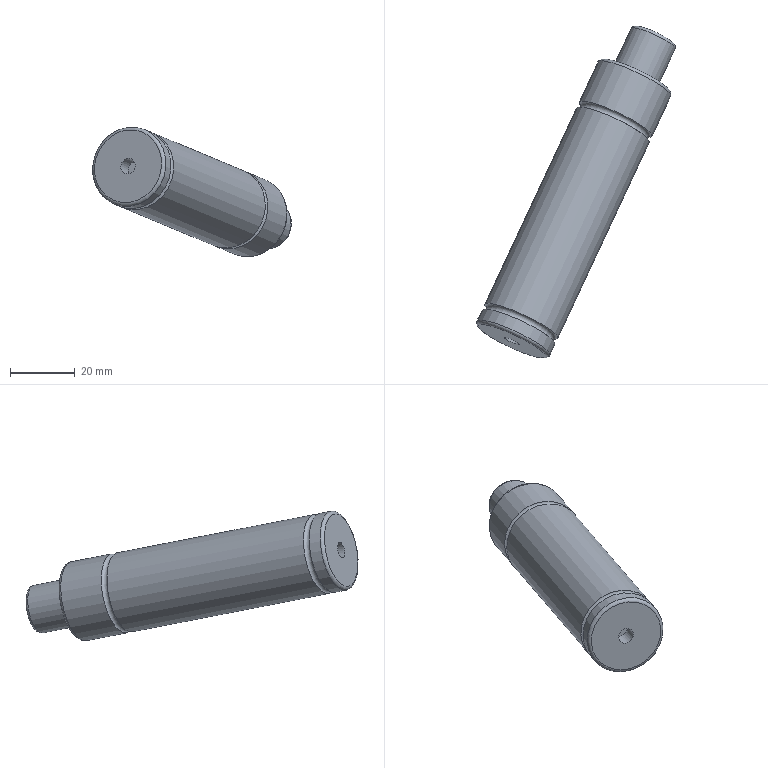Part | NX | features 1 2 | 1 solid | 17 faces | box 61.606 x 102.919 x 40.18 mm | volume 46865 mm3 | cylinder 6 | torus 5 | plane 4 | cone 2 | commonest cylinder face diameters 24.9 x3 2 x1 4.9 x1 15 x1
STEP:
#1=CARTESIAN_POINT('',(294.815,638.267,112.369));
#2=VERTEX_POINT('',#1);
#3=CARTESIAN_POINT('',(283.532,643.529,112.369));
#4=DIRECTION('',(0.4162,0.8925,-0.1736));
#5=DIRECTION('',(0.9063,-0.4226,0.));
#6=AXIS2_PLACEMENT_3D('',#3,#4,#5);
#7=CIRCLE('',#6,12.45);
#8=EDGE_CURVE('',#2,#2,#7,.T.);
#9=ORIENTED_EDGE('',*,*,#8,.T.);
#10=EDGE_LOOP('',(#9));
#11=FACE_BOUND('',#10,.T.);
#12=CARTESIAN_POINT('',(295.648,640.053,112.022));
#13=VERTEX_POINT('',#12);
#14=CARTESIAN_POINT('',(284.364,645.314,112.022));
#15=DIRECTION('',(0.4162,0.8925,-0.1736));
#16=DIRECTION('',(0.9063,-0.4226,0.));
#17=AXIS2_PLACEMENT_3D('',#14,#15,#16);
#18=CIRCLE('',#17,12.45);
#19=EDGE_CURVE('',#13,#13,#18,.T.);
#20=ORIENTED_EDGE('',*,*,#19,.F.);
#21=EDGE_LOOP('',(#20));
#22=FACE_BOUND('',#21,.T.);
#23=CARTESIAN_POINT('',(283.948,644.422,112.195));
#24=DIRECTION('',(0.4162,0.8925,-0.1736));
#25=DIRECTION('',(0.07339,0.1574,0.9848));
#26=AXIS2_PLACEMENT_3D('',#23,#24,#25);
#27=TOROIDAL_SURFACE('',#26,12.45,1.);
#28=ADVANCED_FACE('',(#11,#22),#27,.F.);
#29=CARTESIAN_POINT('',(266.431,577.396,124.212));
#30=VERTEX_POINT('',#29);
#31=CARTESIAN_POINT('',(255.147,582.658,124.212));
#32=DIRECTION('',(0.4162,0.8925,-0.1736));
#33=DIRECTION('',(0.9063,-0.4226,0.));
#34=AXIS2_PLACEMENT_3D('',#31,#32,#33);
#35=CIRCLE('',#34,12.45);
#36=EDGE_CURVE('',#30,#30,#35,.T.);
#37=ORIENTED_EDGE('',*,*,#36,.F.);
#38=EDGE_LOOP('',(#37));
#39=FACE_BOUND('',#38,.T.);
#40=CARTESIAN_POINT('',(265.598,575.611,124.559));
#41=VERTEX_POINT('',#40);
#42=CARTESIAN_POINT('',(254.315,580.873,124.559));
#43=DIRECTION('',(-0.4162,-0.8925,0.1736));
#44=DIRECTION('',(0.9063,-0.4226,0.));
#45=AXIS2_PLACEMENT_3D('',#42,#43,#44);
#46=CIRCLE('',#45,12.45);
#47=EDGE_CURVE('',#41,#41,#46,.T.);
#48=ORIENTED_EDGE('',*,*,#47,.F.);
#49=EDGE_LOOP('',(#48));
#50=FACE_BOUND('',#49,.T.);
#51=CARTESIAN_POINT('',(254.731,581.765,124.386));
#52=DIRECTION('',(0.4162,0.8925,-0.1736));
#53=DIRECTION('',(0.07339,0.1574,0.9848));
#54=AXIS2_PLACEMENT_3D('',#51,#52,#53);
#55=TOROIDAL_SURFACE('',#54,12.45,1.);
#56=ADVANCED_FACE('',(#39,#50),#55,.F.);
#57=CARTESIAN_POINT('',(301.475,652.548,109.591));
#58=VERTEX_POINT('',#57);
#59=CARTESIAN_POINT('',(290.191,657.81,109.591));
#60=DIRECTION('',(0.4162,0.8925,-0.1736));
#61=DIRECTION('',(0.9063,-0.4226,0.));
#62=AXIS2_PLACEMENT_3D('',#59,#60,#61);
#63=CIRCLE('',#62,12.45);
#64=EDGE_CURVE('',#58,#58,#63,.T.);
#65=ORIENTED_EDGE('',*,*,#64,.T.);
#66=EDGE_LOOP('',(#65));
#67=FACE_BOUND('',#66,.T.);
#68=CARTESIAN_POINT('',(300.984,653.863,109.417));
#69=VERTEX_POINT('',#68);
#70=CARTESIAN_POINT('',(290.607,658.702,109.417));
#71=DIRECTION('',(0.4162,0.8925,-0.1736));
#72=DIRECTION('',(0.9063,-0.4226,0.));
#73=AXIS2_PLACEMENT_3D('',#70,#71,#72);
#74=CIRCLE('',#73,11.45);
#75=EDGE_CURVE('',#69,#69,#74,.T.);
#76=ORIENTED_EDGE('',*,*,#75,.F.);
#77=EDGE_LOOP('',(#76));
#78=FACE_BOUND('',#77,.T.);
#79=CARTESIAN_POINT('',(290.191,657.81,109.591));
#80=DIRECTION('',(0.4162,0.8925,-0.1736));
#81=DIRECTION('',(0.07339,0.1574,0.9848));
#82=AXIS2_PLACEMENT_3D('',#79,#80,#81);
#83=TOROIDAL_SURFACE('',#82,11.45,1.);
#84=ADVANCED_FACE('',(#67,#78),#83,.T.);
#85=ORIENTED_EDGE('',*,*,#19,.T.);
#86=EDGE_LOOP('',(#85));
#87=FACE_BOUND('',#86,.T.);
#88=ORIENTED_EDGE('',*,*,#64,.F.);
#89=EDGE_LOOP('',(#88));
#90=FACE_BOUND('',#89,.T.);
#91=CARTESIAN_POINT('',(287.278,651.562,110.806));
#92=DIRECTION('',(-0.4162,-0.8925,0.1736));
#93=DIRECTION('',(-0.07339,-0.1574,-0.9848));
#94=AXIS2_PLACEMENT_3D('',#91,#92,#93);
#95=CYLINDRICAL_SURFACE('',#94,12.45);
#96=ADVANCED_FACE('',(#87,#90),#95,.T.);
#97=ORIENTED_EDGE('',*,*,#36,.T.);
#98=EDGE_LOOP('',(#97));
#99=FACE_BOUND('',#98,.T.);
#100=ORIENTED_EDGE('',*,*,#8,.F.);
#101=EDGE_LOOP('',(#100));
#102=FACE_BOUND('',#101,.T.);
#103=CARTESIAN_POINT('',(268.133,610.505,118.794));
#104=DIRECTION('',(-0.4162,-0.8925,0.1736));
#105=DIRECTION('',(-0.07339,-0.1574,-0.9848));
#106=AXIS2_PLACEMENT_3D('',#103,#104,#105);
#107=CYLINDRICAL_SURFACE('',#106,12.45);
#108=ADVANCED_FACE('',(#99,#102),#107,.T.);
#109=CARTESIAN_POINT('',(262.694,571.75,125.393));
#110=VERTEX_POINT('',#109);
#111=CARTESIAN_POINT('',(252.317,576.589,125.393));
#112=DIRECTION('',(0.4162,0.8925,-0.1736));
#113=DIRECTION('',(0.9063,-0.4226,0.));
#114=AXIS2_PLACEMENT_3D('',#111,#112,#113);
#115=CIRCLE('',#114,11.45);
#116=EDGE_CURVE('',#110,#110,#115,.T.);
#117=ORIENTED_EDGE('',*,*,#116,.T.);
#118=EDGE_LOOP('',(#117));
#119=FACE_BOUND('',#118,.T.);
#120=CARTESIAN_POINT('',(264.017,572.22,125.219));
#121=VERTEX_POINT('',#120);
#122=CARTESIAN_POINT('',(252.733,577.481,125.219));
#123=DIRECTION('',(0.4162,0.8925,-0.1736));
#124=DIRECTION('',(0.9063,-0.4226,0.));
#125=AXIS2_PLACEMENT_3D('',#122,#123,#124);
#126=CIRCLE('',#125,12.45);
#127=EDGE_CURVE('',#121,#121,#126,.T.);
#128=ORIENTED_EDGE('',*,*,#127,.F.);
#129=EDGE_LOOP('',(#128));
#130=FACE_BOUND('',#129,.T.);
#131=CARTESIAN_POINT('',(252.733,577.481,125.219));
#132=DIRECTION('',(0.4162,0.8925,-0.1736));
#133=DIRECTION('',(0.07339,0.1574,0.9848));
#134=AXIS2_PLACEMENT_3D('',#131,#132,#133);
#135=TOROIDAL_SURFACE('',#134,11.45,1.);
#136=ADVANCED_FACE('',(#119,#130),#135,.T.);
#137=ORIENTED_EDGE('',*,*,#127,.T.);
#138=EDGE_LOOP('',(#137));
#139=FACE_BOUND('',#138,.T.);
#140=ORIENTED_EDGE('',*,*,#47,.T.);
#141=EDGE_LOOP('',(#140));
#142=FACE_BOUND('',#141,.T.);
#143=CARTESIAN_POINT('',(268.133,610.505,118.794));
#144=DIRECTION('',(-0.4162,-0.8925,0.1736));
#145=DIRECTION('',(-0.07339,-0.1574,-0.9848));
#146=AXIS2_PLACEMENT_3D('',#143,#144,#145);
#147=CYLINDRICAL_SURFACE('',#146,12.45);
#148=ADVANCED_FACE('',(#139,#142),#147,.T.);
#149=CARTESIAN_POINT('',(302.815,667.136,107.16));
#150=VERTEX_POINT('',#149);
#151=CARTESIAN_POINT('',(296.018,670.305,107.16));
#152=DIRECTION('',(0.4162,0.8925,-0.1736));
#153=DIRECTION('',(0.9063,-0.4226,0.));
#154=AXIS2_PLACEMENT_3D('',#151,#152,#153);
#155=CIRCLE('',#154,7.5);
#156=EDGE_CURVE('',#150,#150,#155,.T.);
#157=ORIENTED_EDGE('',*,*,#156,.T.);
#158=EDGE_LOOP('',(#157));
#159=FACE_BOUND('',#158,.T.);
#160=CARTESIAN_POINT('',(302.325,668.451,106.986));
#161=VERTEX_POINT('',#160);
#162=CARTESIAN_POINT('',(296.434,671.198,106.986));
#163=DIRECTION('',(0.4162,0.8925,-0.1736));
#164=DIRECTION('',(0.9063,-0.4226,0.));
#165=AXIS2_PLACEMENT_3D('',#162,#163,#164);
#166=CIRCLE('',#165,6.5);
#167=EDGE_CURVE('',#161,#161,#166,.T.);
#168=ORIENTED_EDGE('',*,*,#167,.F.);
#169=EDGE_LOOP('',(#168));
#170=FACE_BOUND('',#169,.T.);
#171=CARTESIAN_POINT('',(296.018,670.305,107.16));
#172=DIRECTION('',(0.4162,0.8925,-0.1736));
#173=DIRECTION('',(0.07339,0.1574,0.9848));
#174=AXIS2_PLACEMENT_3D('',#171,#172,#173);
#175=TOROIDAL_SURFACE('',#174,6.5,1.);
#176=ADVANCED_FACE('',(#159,#170),#175,.T.);
#177=CARTESIAN_POINT('',(297.405,655.533,109.417));
#178=VERTEX_POINT('',#177);
#179=CARTESIAN_POINT('',(290.607,658.702,109.417));
#180=DIRECTION('',(-0.4162,-0.8925,0.1736));
#181=DIRECTION('',(0.9063,-0.4226,0.));
#182=AXIS2_PLACEMENT_3D('',#179,#180,#181);
#183=CIRCLE('',#182,7.5);
#184=EDGE_CURVE('',#178,#178,#183,.T.);
#185=ORIENTED_EDGE('',*,*,#184,.F.);
#186=EDGE_LOOP('',(#185));
#187=FACE_BOUND('',#186,.T.);
#188=ORIENTED_EDGE('',*,*,#156,.F.);
#189=EDGE_LOOP('',(#188));
#190=FACE_BOUND('',#189,.T.);
#191=CARTESIAN_POINT('',(293.313,664.504,108.288));
#192=DIRECTION('',(-0.4162,-0.8925,0.1736));
#193=DIRECTION('',(-0.07339,-0.1574,-0.9848));
#194=AXIS2_PLACEMENT_3D('',#191,#192,#193);
#195=CYLINDRICAL_SURFACE('',#194,7.5);
#196=ADVANCED_FACE('',(#187,#190),#195,.T.);
#197=CARTESIAN_POINT('',(298.247,670.353,106.986));
#198=VERTEX_POINT('',#197);
#199=CARTESIAN_POINT('',(296.434,671.198,106.986));
#200=DIRECTION('',(-0.4162,-0.8925,0.1736));
#201=DIRECTION('',(0.9063,-0.4226,0.));
#202=AXIS2_PLACEMENT_3D('',#199,#200,#201);
#203=CIRCLE('',#202,2.);
#204=EDGE_CURVE('',#198,#198,#203,.T.);
#205=ORIENTED_EDGE('',*,*,#204,.F.);
#206=EDGE_LOOP('',(#205));
#207=FACE_BOUND('',#206,.T.);
#208=CARTESIAN_POINT('',(296.619,669.229,107.287));
#209=VERTEX_POINT('',#208);
#210=CARTESIAN_POINT('',(295.713,669.652,107.287));
#211=DIRECTION('',(0.4162,0.8925,-0.1736));
#212=DIRECTION('',(0.9063,-0.4226,0.));
#213=AXIS2_PLACEMENT_3D('',#210,#211,#212);
#214=CIRCLE('',#213,1.);
#215=EDGE_CURVE('',#209,#209,#214,.T.);
#216=ORIENTED_EDGE('',*,*,#215,.F.);
#217=EDGE_LOOP('',(#216));
#218=FACE_BOUND('',#217,.T.);
#219=CARTESIAN_POINT('',(296.074,670.425,107.136));
#220=DIRECTION('',(0.4162,0.8925,-0.1736));
#221=DIRECTION('',(0.07339,0.1574,0.9848));
#222=AXIS2_PLACEMENT_3D('',#219,#220,#221);
#223=CONICAL_SURFACE('',#222,1.5,0.5236);
#224=ADVANCED_FACE('',(#207,#218),#223,.F.);
#225=ORIENTED_EDGE('',*,*,#215,.T.);
#226=EDGE_LOOP('',(#225));
#227=FACE_BOUND('',#226,.T.);
#228=CARTESIAN_POINT('',(295.051,665.866,107.941));
#229=VERTEX_POINT('',#228);
#230=CARTESIAN_POINT('',(294.145,666.289,107.941));
#231=DIRECTION('',(0.4162,0.8925,-0.1736));
#232=DIRECTION('',(0.9063,-0.4226,0.));
#233=AXIS2_PLACEMENT_3D('',#230,#231,#232);
#234=CIRCLE('',#233,1.);
#235=EDGE_CURVE('',#229,#229,#234,.T.);
#236=ORIENTED_EDGE('',*,*,#235,.F.);
#237=EDGE_LOOP('',(#236));
#238=FACE_BOUND('',#237,.T.);
#239=CARTESIAN_POINT('',(294.929,667.97,107.614));
#240=DIRECTION('',(-0.4162,-0.8925,0.1736));
#241=DIRECTION('',(-0.07339,-0.1574,-0.9848));
#242=AXIS2_PLACEMENT_3D('',#239,#240,#241);
#243=CYLINDRICAL_SURFACE('',#242,1.);
#244=ADVANCED_FACE('',(#227,#238),#243,.F.);
#245=CARTESIAN_POINT('',(293.937,665.843,108.028));
#246=VERTEX_POINT('',#245);
#247=VERTEX_LOOP('',#246);
#248=FACE_BOUND('',#247,.T.);
#249=ORIENTED_EDGE('',*,*,#235,.T.);
#250=EDGE_LOOP('',(#249));
#251=FACE_BOUND('',#250,.T.);
#252=CARTESIAN_POINT('',(294.041,666.066,107.984));
#253=DIRECTION('',(0.4162,0.8925,-0.1736));
#254=DIRECTION('',(0.07339,0.1574,0.9848));
#255=AXIS2_PLACEMENT_3D('',#252,#253,#254);
#256=CONICAL_SURFACE('',#255,0.5,1.107);
#257=ADVANCED_FACE('',(#248,#251),#256,.F.);
#258=CARTESIAN_POINT('',(256.827,580.462,124.438));
#259=VERTEX_POINT('',#258);
#260=CARTESIAN_POINT('',(254.606,581.498,124.438));
#261=DIRECTION('',(-0.4162,-0.8925,0.1736));
#262=DIRECTION('',(0.9063,-0.4226,0.));
#263=AXIS2_PLACEMENT_3D('',#260,#261,#262);
#264=CIRCLE('',#263,2.45);
#265=EDGE_CURVE('',#259,#259,#264,.T.);
#266=ORIENTED_EDGE('',*,*,#265,.F.);
#267=EDGE_LOOP('',(#266));
#268=FACE_BOUND('',#267,.T.);
#269=CARTESIAN_POINT('',(254.537,575.553,125.393));
#270=VERTEX_POINT('',#269);
#271=CARTESIAN_POINT('',(252.317,576.589,125.393));
#272=DIRECTION('',(0.4162,0.8925,-0.1736));
#273=DIRECTION('',(0.9063,-0.4226,0.));
#274=AXIS2_PLACEMENT_3D('',#271,#272,#273);
#275=CIRCLE('',#274,2.45);
#276=EDGE_CURVE('',#270,#270,#275,.T.);
#277=ORIENTED_EDGE('',*,*,#276,.F.);
#278=EDGE_LOOP('',(#277));
#279=FACE_BOUND('',#278,.T.);
#280=CARTESIAN_POINT('',(252.317,576.589,125.393));
#281=DIRECTION('',(-0.4162,-0.8925,0.1736));
#282=DIRECTION('',(-0.07339,-0.1574,-0.9848));
#283=AXIS2_PLACEMENT_3D('',#280,#281,#282);
#284=CYLINDRICAL_SURFACE('',#283,2.45);
#285=ADVANCED_FACE('',(#268,#279),#284,.F.);
#286=ORIENTED_EDGE('',*,*,#265,.T.);
#287=EDGE_LOOP('',(#286));
#288=FACE_BOUND('',#287,.T.);
#289=CARTESIAN_POINT('',(254.606,581.498,124.438));
#290=DIRECTION('',(-0.4162,-0.8925,0.1736));
#291=DIRECTION('',(-0.07339,-0.1574,-0.9848));
#292=AXIS2_PLACEMENT_3D('',#289,#290,#291);
#293=PLANE('',#292);
#294=ADVANCED_FACE('',(#288),#293,.T.);
#295=ORIENTED_EDGE('',*,*,#204,.T.);
#296=EDGE_LOOP('',(#295));
#297=FACE_BOUND('',#296,.T.);
#298=ORIENTED_EDGE('',*,*,#167,.T.);
#299=EDGE_LOOP('',(#298));
#300=FACE_BOUND('',#299,.T.);
#301=CARTESIAN_POINT('',(299.379,669.824,106.986));
#302=DIRECTION('',(0.4162,0.8925,-0.1736));
#303=DIRECTION('',(0.07339,0.1574,0.9848));
#304=AXIS2_PLACEMENT_3D('',#301,#302,#303);
#305=PLANE('',#304);
#306=ADVANCED_FACE('',(#297,#300),#305,.T.);
#307=ORIENTED_EDGE('',*,*,#276,.T.);
#308=EDGE_LOOP('',(#307));
#309=FACE_BOUND('',#308,.T.);
#310=ORIENTED_EDGE('',*,*,#116,.F.);
#311=EDGE_LOOP('',(#310));
#312=FACE_BOUND('',#311,.T.);
#313=CARTESIAN_POINT('',(257.506,574.169,125.393));
#314=DIRECTION('',(-0.4162,-0.8925,0.1736));
#315=DIRECTION('',(0.9063,-0.4226,0.));
#316=AXIS2_PLACEMENT_3D('',#313,#314,#315);
#317=PLANE('',#316);
#318=ADVANCED_FACE('',(#309,#312),#317,.T.);
#319=ORIENTED_EDGE('',*,*,#184,.T.);
#320=EDGE_LOOP('',(#319));
#321=FACE_BOUND('',#320,.T.);
#322=ORIENTED_EDGE('',*,*,#75,.T.);
#323=EDGE_LOOP('',(#322));
#324=FACE_BOUND('',#323,.T.);
#325=CARTESIAN_POINT('',(295.796,656.283,109.417));
#326=DIRECTION('',(0.4162,0.8925,-0.1736));
#327=DIRECTION('',(0.07339,0.1574,0.9848));
#328=AXIS2_PLACEMENT_3D('',#325,#326,#327);
#329=PLANE('',#328);
#330=ADVANCED_FACE('',(#321,#324),#329,.T.);
#331=CLOSED_SHELL('',(#28,#56,#84,#96,#108,#136,#148,#176,#196,#224,#244,#257,#285,#294,#306,#318,#330));
#332=MANIFOLD_SOLID_BREP('',#331);
#333=(LENGTH_UNIT()NAMED_UNIT(*)SI_UNIT(.MILLI.,.METRE.));
#334=UNCERTAINTY_MEASURE_WITH_UNIT(LENGTH_MEASURE(0.00001),#333,'','');
#335=(NAMED_UNIT(*)PLANE_ANGLE_UNIT()SI_UNIT($,.RADIAN.));
#336=(NAMED_UNIT(*)SI_UNIT($,.STERADIAN.)SOLID_ANGLE_UNIT());
#337=(GEOMETRIC_REPRESENTATION_CONTEXT(3)GLOBAL_UNCERTAINTY_ASSIGNED_CONTEXT((#334))GLOBAL_UNIT_ASSIGNED_CONTEXT((#333,#335,#336))REPRESENTATION_CONTEXT('',''));
#338=ADVANCED_BREP_SHAPE_REPRESENTATION('',(#332),#337);